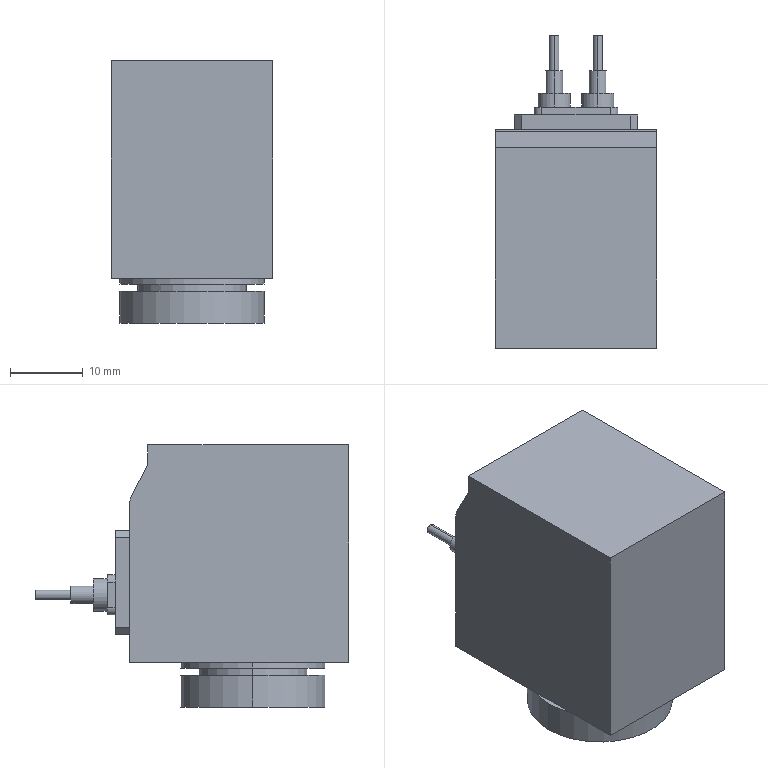Part | SolidWorks | features BaseBody 1 | 1 solid | 54 faces | box 22.3 x 43.2 x 36.2 mm | volume 22382 mm3 | plane 31 | cylinder 23 | commonest cylinder face diameters 1.3 x4 2 x4 2.4 x4 4.5 x4 20 x4 15 x2
STEP:
#1=CARTESIAN_POINT('',(-10.,0.,-31.8));
#2=VERTEX_POINT('',#1);
#3=CARTESIAN_POINT('',(10.,0.,-31.8));
#4=VERTEX_POINT('',#3);
#5=CARTESIAN_POINT('',(0.,0.,-31.8));
#6=DIRECTION('',(0.,0.,-1.));
#7=DIRECTION('',(-1.,0.,0.));
#8=AXIS2_PLACEMENT_3D('',#5,#6,#7);
#9=CIRCLE('',#8,10.);
#10=EDGE_CURVE('',#2,#4,#9,.T.);
#11=ORIENTED_EDGE('',*,*,#10,.T.);
#12=CARTESIAN_POINT('',(10.,0.,-36.2));
#13=VERTEX_POINT('',#12);
#14=CARTESIAN_POINT('',(10.,0.,-36.2));
#15=DIRECTION('',(0.,0.,-1.));
#16=VECTOR('',#15,1000.);
#17=LINE('',#14,#16);
#18=EDGE_CURVE('',#4,#13,#17,.T.);
#19=ORIENTED_EDGE('',*,*,#18,.T.);
#20=CARTESIAN_POINT('',(-10.,0.,-36.2));
#21=VERTEX_POINT('',#20);
#22=CARTESIAN_POINT('',(0.,0.,-36.2));
#23=DIRECTION('',(0.,0.,-1.));
#24=DIRECTION('',(-1.,0.,0.));
#25=AXIS2_PLACEMENT_3D('',#22,#23,#24);
#26=CIRCLE('',#25,10.);
#27=EDGE_CURVE('',#21,#13,#26,.T.);
#28=ORIENTED_EDGE('',*,*,#27,.F.);
#29=CARTESIAN_POINT('',(-10.,0.,-36.2));
#30=DIRECTION('',(0.,0.,-1.));
#31=VECTOR('',#30,1000.);
#32=LINE('',#29,#31);
#33=EDGE_CURVE('',#2,#21,#32,.T.);
#34=ORIENTED_EDGE('',*,*,#33,.F.);
#35=EDGE_LOOP('',(#11,#19,#28,#34));
#36=FACE_OUTER_BOUND('',#35,.T.);
#37=CARTESIAN_POINT('',(0.,0.,-36.2));
#38=DIRECTION('',(0.,0.,-1.));
#39=DIRECTION('',(-1.,0.,0.));
#40=AXIS2_PLACEMENT_3D('',#37,#38,#39);
#41=CYLINDRICAL_SURFACE('',#40,10.);
#42=ADVANCED_FACE('',(#36),#41,.T.);
#43=CARTESIAN_POINT('',(-3.,30.,-20.05));
#44=VERTEX_POINT('',#43);
#45=CARTESIAN_POINT('',(-3.,30.,-21.35));
#46=VERTEX_POINT('',#45);
#47=CARTESIAN_POINT('',(-3.,30.,-20.7));
#48=DIRECTION('',(0.,1.,0.));
#49=DIRECTION('',(1.,0.,0.));
#50=AXIS2_PLACEMENT_3D('',#47,#48,#49);
#51=CIRCLE('',#50,0.65);
#52=EDGE_CURVE('',#44,#46,#51,.T.);
#53=ORIENTED_EDGE('',*,*,#52,.F.);
#54=CARTESIAN_POINT('',(-3.,25.1,-20.05));
#55=VERTEX_POINT('',#54);
#56=CARTESIAN_POINT('',(-3.,30.,-20.05));
#57=DIRECTION('',(0.,-1.,0.));
#58=VECTOR('',#57,1000.);
#59=LINE('',#56,#58);
#60=EDGE_CURVE('',#44,#55,#59,.T.);
#61=ORIENTED_EDGE('',*,*,#60,.T.);
#62=CARTESIAN_POINT('',(-3.,25.1,-21.35));
#63=VERTEX_POINT('',#62);
#64=CARTESIAN_POINT('',(-3.,25.1,-20.7));
#65=DIRECTION('',(0.,1.,0.));
#66=DIRECTION('',(1.,0.,0.));
#67=AXIS2_PLACEMENT_3D('',#64,#65,#66);
#68=CIRCLE('',#67,0.65);
#69=EDGE_CURVE('',#55,#63,#68,.T.);
#70=ORIENTED_EDGE('',*,*,#69,.T.);
#71=CARTESIAN_POINT('',(-3.,30.,-21.35));
#72=DIRECTION('',(0.,-1.,0.));
#73=VECTOR('',#72,1000.);
#74=LINE('',#71,#73);
#75=EDGE_CURVE('',#46,#63,#74,.T.);
#76=ORIENTED_EDGE('',*,*,#75,.F.);
#77=EDGE_LOOP('',(#53,#61,#70,#76));
#78=FACE_OUTER_BOUND('',#77,.T.);
#79=CARTESIAN_POINT('',(-3.,30.,-20.7));
#80=DIRECTION('',(0.,-1.,0.));
#81=DIRECTION('',(0.,0.,-1.));
#82=AXIS2_PLACEMENT_3D('',#79,#80,#81);
#83=CYLINDRICAL_SURFACE('',#82,0.65);
#84=ADVANCED_FACE('',(#78),#83,.T.);
#85=CARTESIAN_POINT('',(3.,30.,-20.05));
#86=VERTEX_POINT('',#85);
#87=CARTESIAN_POINT('',(3.,30.,-21.35));
#88=VERTEX_POINT('',#87);
#89=CARTESIAN_POINT('',(3.,30.,-20.7));
#90=DIRECTION('',(0.,1.,0.));
#91=DIRECTION('',(1.,0.,0.));
#92=AXIS2_PLACEMENT_3D('',#89,#90,#91);
#93=CIRCLE('',#92,0.65);
#94=EDGE_CURVE('',#86,#88,#93,.T.);
#95=ORIENTED_EDGE('',*,*,#94,.F.);
#96=CARTESIAN_POINT('',(3.,25.1,-20.05));
#97=VERTEX_POINT('',#96);
#98=CARTESIAN_POINT('',(3.,30.,-20.05));
#99=DIRECTION('',(0.,-1.,0.));
#100=VECTOR('',#99,1000.);
#101=LINE('',#98,#100);
#102=EDGE_CURVE('',#86,#97,#101,.T.);
#103=ORIENTED_EDGE('',*,*,#102,.T.);
#104=CARTESIAN_POINT('',(3.,25.1,-21.35));
#105=VERTEX_POINT('',#104);
#106=CARTESIAN_POINT('',(3.,25.1,-20.7));
#107=DIRECTION('',(0.,1.,0.));
#108=DIRECTION('',(1.,0.,0.));
#109=AXIS2_PLACEMENT_3D('',#106,#107,#108);
#110=CIRCLE('',#109,0.65);
#111=EDGE_CURVE('',#97,#105,#110,.T.);
#112=ORIENTED_EDGE('',*,*,#111,.T.);
#113=CARTESIAN_POINT('',(3.,30.,-21.35));
#114=DIRECTION('',(0.,-1.,0.));
#115=VECTOR('',#114,1000.);
#116=LINE('',#113,#115);
#117=EDGE_CURVE('',#88,#105,#116,.T.);
#118=ORIENTED_EDGE('',*,*,#117,.F.);
#119=EDGE_LOOP('',(#95,#103,#112,#118));
#120=FACE_OUTER_BOUND('',#119,.T.);
#121=CARTESIAN_POINT('',(3.,30.,-20.7));
#122=DIRECTION('',(0.,-1.,0.));
#123=DIRECTION('',(0.,0.,-1.));
#124=AXIS2_PLACEMENT_3D('',#121,#122,#123);
#125=CYLINDRICAL_SURFACE('',#124,0.65);
#126=ADVANCED_FACE('',(#120),#125,.T.);
#127=CARTESIAN_POINT('',(-7.5,0.,-30.8));
#128=VERTEX_POINT('',#127);
#129=CARTESIAN_POINT('',(7.5,0.,-30.8));
#130=VERTEX_POINT('',#129);
#131=CARTESIAN_POINT('',(0.,0.,-30.8));
#132=DIRECTION('',(0.,0.,-1.));
#133=DIRECTION('',(-1.,0.,0.));
#134=AXIS2_PLACEMENT_3D('',#131,#132,#133);
#135=CIRCLE('',#134,7.5);
#136=EDGE_CURVE('',#128,#130,#135,.T.);
#137=ORIENTED_EDGE('',*,*,#136,.T.);
#138=CARTESIAN_POINT('',(7.5,0.,-31.8));
#139=VERTEX_POINT('',#138);
#140=CARTESIAN_POINT('',(7.5,0.,-36.2));
#141=DIRECTION('',(0.,0.,-1.));
#142=VECTOR('',#141,1000.);
#143=LINE('',#140,#142);
#144=EDGE_CURVE('',#130,#139,#143,.T.);
#145=ORIENTED_EDGE('',*,*,#144,.T.);
#146=CARTESIAN_POINT('',(-7.5,0.,-31.8));
#147=VERTEX_POINT('',#146);
#148=CARTESIAN_POINT('',(0.,0.,-31.8));
#149=DIRECTION('',(0.,0.,-1.));
#150=DIRECTION('',(-1.,0.,0.));
#151=AXIS2_PLACEMENT_3D('',#148,#149,#150);
#152=CIRCLE('',#151,7.5);
#153=EDGE_CURVE('',#147,#139,#152,.T.);
#154=ORIENTED_EDGE('',*,*,#153,.F.);
#155=CARTESIAN_POINT('',(-7.5,0.,-36.2));
#156=DIRECTION('',(0.,0.,-1.));
#157=VECTOR('',#156,1000.);
#158=LINE('',#155,#157);
#159=EDGE_CURVE('',#128,#147,#158,.T.);
#160=ORIENTED_EDGE('',*,*,#159,.F.);
#161=EDGE_LOOP('',(#137,#145,#154,#160));
#162=FACE_OUTER_BOUND('',#161,.T.);
#163=CARTESIAN_POINT('',(0.,0.,-36.2));
#164=DIRECTION('',(0.,0.,-1.));
#165=DIRECTION('',(-1.,0.,0.));
#166=AXIS2_PLACEMENT_3D('',#163,#164,#165);
#167=CYLINDRICAL_SURFACE('',#166,7.5);
#168=ADVANCED_FACE('',(#162),#167,.T.);
#169=CARTESIAN_POINT('',(-3.,25.1,-19.5));
#170=VERTEX_POINT('',#169);
#171=CARTESIAN_POINT('',(-3.,25.1,-21.9));
#172=VERTEX_POINT('',#171);
#173=CARTESIAN_POINT('',(-3.,25.1,-20.7));
#174=DIRECTION('',(0.,1.,0.));
#175=DIRECTION('',(1.,0.,0.));
#176=AXIS2_PLACEMENT_3D('',#173,#174,#175);
#177=CIRCLE('',#176,1.2);
#178=EDGE_CURVE('',#170,#172,#177,.T.);
#179=ORIENTED_EDGE('',*,*,#178,.F.);
#180=CARTESIAN_POINT('',(-3.,22.,-19.5));
#181=VERTEX_POINT('',#180);
#182=CARTESIAN_POINT('',(-3.,25.1,-19.5));
#183=DIRECTION('',(0.,-1.,0.));
#184=VECTOR('',#183,1000.);
#185=LINE('',#182,#184);
#186=EDGE_CURVE('',#170,#181,#185,.T.);
#187=ORIENTED_EDGE('',*,*,#186,.T.);
#188=CARTESIAN_POINT('',(-3.,22.,-21.9));
#189=VERTEX_POINT('',#188);
#190=CARTESIAN_POINT('',(-3.,22.,-20.7));
#191=DIRECTION('',(0.,-1.,0.));
#192=DIRECTION('',(0.,0.,1.));
#193=AXIS2_PLACEMENT_3D('',#190,#191,#192);
#194=CIRCLE('',#193,1.2);
#195=EDGE_CURVE('',#189,#181,#194,.T.);
#196=ORIENTED_EDGE('',*,*,#195,.F.);
#197=CARTESIAN_POINT('',(-3.,25.1,-21.9));
#198=DIRECTION('',(0.,-1.,0.));
#199=VECTOR('',#198,1000.);
#200=LINE('',#197,#199);
#201=EDGE_CURVE('',#172,#189,#200,.T.);
#202=ORIENTED_EDGE('',*,*,#201,.F.);
#203=EDGE_LOOP('',(#179,#187,#196,#202));
#204=FACE_OUTER_BOUND('',#203,.T.);
#205=CARTESIAN_POINT('',(-3.,25.1,-20.7));
#206=DIRECTION('',(0.,-1.,0.));
#207=DIRECTION('',(0.,0.,-1.));
#208=AXIS2_PLACEMENT_3D('',#205,#206,#207);
#209=CYLINDRICAL_SURFACE('',#208,1.2);
#210=ADVANCED_FACE('',(#204),#209,.T.);
#211=CARTESIAN_POINT('',(3.,25.1,-19.5));
#212=VERTEX_POINT('',#211);
#213=CARTESIAN_POINT('',(3.,25.1,-21.9));
#214=VERTEX_POINT('',#213);
#215=CARTESIAN_POINT('',(3.,25.1,-20.7));
#216=DIRECTION('',(0.,1.,0.));
#217=DIRECTION('',(1.,0.,0.));
#218=AXIS2_PLACEMENT_3D('',#215,#216,#217);
#219=CIRCLE('',#218,1.2);
#220=EDGE_CURVE('',#212,#214,#219,.T.);
#221=ORIENTED_EDGE('',*,*,#220,.F.);
#222=CARTESIAN_POINT('',(3.,22.,-19.5));
#223=VERTEX_POINT('',#222);
#224=CARTESIAN_POINT('',(3.,25.1,-19.5));
#225=DIRECTION('',(0.,-1.,0.));
#226=VECTOR('',#225,1000.);
#227=LINE('',#224,#226);
#228=EDGE_CURVE('',#212,#223,#227,.T.);
#229=ORIENTED_EDGE('',*,*,#228,.T.);
#230=CARTESIAN_POINT('',(3.,22.,-21.9));
#231=VERTEX_POINT('',#230);
#232=CARTESIAN_POINT('',(3.,22.,-20.7));
#233=DIRECTION('',(0.,-1.,0.));
#234=DIRECTION('',(0.,0.,1.));
#235=AXIS2_PLACEMENT_3D('',#232,#233,#234);
#236=CIRCLE('',#235,1.2);
#237=EDGE_CURVE('',#231,#223,#236,.T.);
#238=ORIENTED_EDGE('',*,*,#237,.F.);
#239=CARTESIAN_POINT('',(3.,25.1,-21.9));
#240=DIRECTION('',(0.,-1.,0.));
#241=VECTOR('',#240,1000.);
#242=LINE('',#239,#241);
#243=EDGE_CURVE('',#214,#231,#242,.T.);
#244=ORIENTED_EDGE('',*,*,#243,.F.);
#245=EDGE_LOOP('',(#221,#229,#238,#244));
#246=FACE_OUTER_BOUND('',#245,.T.);
#247=CARTESIAN_POINT('',(3.,25.1,-20.7));
#248=DIRECTION('',(0.,-1.,0.));
#249=DIRECTION('',(0.,0.,-1.));
#250=AXIS2_PLACEMENT_3D('',#247,#248,#249);
#251=CYLINDRICAL_SURFACE('',#250,1.2);
#252=ADVANCED_FACE('',(#246),#251,.T.);
#253=CARTESIAN_POINT('',(-10.,0.,-30.));
#254=VERTEX_POINT('',#253);
#255=CARTESIAN_POINT('',(10.,0.,-30.));
#256=VERTEX_POINT('',#255);
#257=CARTESIAN_POINT('',(0.,0.,-30.));
#258=DIRECTION('',(0.,0.,-1.));
#259=DIRECTION('',(1.,0.,0.));
#260=AXIS2_PLACEMENT_3D('',#257,#258,#259);
#261=CIRCLE('',#260,10.);
#262=EDGE_CURVE('',#254,#256,#261,.T.);
#263=ORIENTED_EDGE('',*,*,#262,.T.);
#264=CARTESIAN_POINT('',(10.,0.,-30.8));
#265=VERTEX_POINT('',#264);
#266=CARTESIAN_POINT('',(10.,0.,-36.2));
#267=DIRECTION('',(0.,0.,-1.));
#268=VECTOR('',#267,1000.);
#269=LINE('',#266,#268);
#270=EDGE_CURVE('',#256,#265,#269,.T.);
#271=ORIENTED_EDGE('',*,*,#270,.T.);
#272=CARTESIAN_POINT('',(-10.,0.,-30.8));
#273=VERTEX_POINT('',#272);
#274=CARTESIAN_POINT('',(0.,0.,-30.8));
#275=DIRECTION('',(0.,0.,-1.));
#276=DIRECTION('',(-1.,0.,0.));
#277=AXIS2_PLACEMENT_3D('',#274,#275,#276);
#278=CIRCLE('',#277,10.);
#279=EDGE_CURVE('',#273,#265,#278,.T.);
#280=ORIENTED_EDGE('',*,*,#279,.F.);
#281=CARTESIAN_POINT('',(-10.,0.,-36.2));
#282=DIRECTION('',(0.,0.,-1.));
#283=VECTOR('',#282,1000.);
#284=LINE('',#281,#283);
#285=EDGE_CURVE('',#254,#273,#284,.T.);
#286=ORIENTED_EDGE('',*,*,#285,.F.);
#287=EDGE_LOOP('',(#263,#271,#280,#286));
#288=FACE_OUTER_BOUND('',#287,.T.);
#289=CARTESIAN_POINT('',(0.,0.,-36.2));
#290=DIRECTION('',(0.,0.,-1.));
#291=DIRECTION('',(-1.,0.,0.));
#292=AXIS2_PLACEMENT_3D('',#289,#290,#291);
#293=CYLINDRICAL_SURFACE('',#292,10.);
#294=ADVANCED_FACE('',(#288),#293,.T.);
#295=CARTESIAN_POINT('',(-3.,22.,-18.45));
#296=VERTEX_POINT('',#295);
#297=CARTESIAN_POINT('',(-3.,22.,-22.95));
#298=VERTEX_POINT('',#297);
#299=CARTESIAN_POINT('',(-3.,22.,-20.7));
#300=DIRECTION('',(0.,1.,0.));
#301=DIRECTION('',(1.,0.,0.));
#302=AXIS2_PLACEMENT_3D('',#299,#300,#301);
#303=CIRCLE('',#302,2.25);
#304=EDGE_CURVE('',#296,#298,#303,.T.);
#305=ORIENTED_EDGE('',*,*,#304,.F.);
#306=CARTESIAN_POINT('',(-3.,20.1,-18.45));
#307=VERTEX_POINT('',#306);
#308=CARTESIAN_POINT('',(-3.,22.,-18.45));
#309=DIRECTION('',(0.,-1.,0.));
#310=VECTOR('',#309,1000.);
#311=LINE('',#308,#310);
#312=EDGE_CURVE('',#296,#307,#311,.T.);
#313=ORIENTED_EDGE('',*,*,#312,.T.);
#314=CARTESIAN_POINT('',(-3.,20.1,-22.95));
#315=VERTEX_POINT('',#314);
#316=CARTESIAN_POINT('',(-3.,20.1,-20.7));
#317=DIRECTION('',(0.,1.,0.));
#318=DIRECTION('',(1.,0.,0.));
#319=AXIS2_PLACEMENT_3D('',#316,#317,#318);
#320=CIRCLE('',#319,2.25);
#321=EDGE_CURVE('',#307,#315,#320,.T.);
#322=ORIENTED_EDGE('',*,*,#321,.T.);
#323=CARTESIAN_POINT('',(-3.,22.,-22.95));
#324=DIRECTION('',(0.,-1.,0.));
#325=VECTOR('',#324,1000.);
#326=LINE('',#323,#325);
#327=EDGE_CURVE('',#298,#315,#326,.T.);
#328=ORIENTED_EDGE('',*,*,#327,.F.);
#329=EDGE_LOOP('',(#305,#313,#322,#328));
#330=FACE_OUTER_BOUND('',#329,.T.);
#331=CARTESIAN_POINT('',(-3.,22.,-20.7));
#332=DIRECTION('',(0.,-1.,0.));
#333=DIRECTION('',(0.,0.,-1.));
#334=AXIS2_PLACEMENT_3D('',#331,#332,#333);
#335=CYLINDRICAL_SURFACE('',#334,2.25);
#336=ADVANCED_FACE('',(#330),#335,.T.);
#337=CARTESIAN_POINT('',(3.,22.,-18.45));
#338=VERTEX_POINT('',#337);
#339=CARTESIAN_POINT('',(3.,22.,-22.95));
#340=VERTEX_POINT('',#339);
#341=CARTESIAN_POINT('',(3.,22.,-20.7));
#342=DIRECTION('',(0.,1.,0.));
#343=DIRECTION('',(1.,0.,0.));
#344=AXIS2_PLACEMENT_3D('',#341,#342,#343);
#345=CIRCLE('',#344,2.25);
#346=EDGE_CURVE('',#338,#340,#345,.T.);
#347=ORIENTED_EDGE('',*,*,#346,.F.);
#348=CARTESIAN_POINT('',(3.,20.1,-18.45));
#349=VERTEX_POINT('',#348);
#350=CARTESIAN_POINT('',(3.,22.,-18.45));
#351=DIRECTION('',(0.,-1.,0.));
#352=VECTOR('',#351,1000.);
#353=LINE('',#350,#352);
#354=EDGE_CURVE('',#338,#349,#353,.T.);
#355=ORIENTED_EDGE('',*,*,#354,.T.);
#356=CARTESIAN_POINT('',(3.,20.1,-22.95));
#357=VERTEX_POINT('',#356);
#358=CARTESIAN_POINT('',(3.,20.1,-20.7));
#359=DIRECTION('',(0.,1.,0.));
#360=DIRECTION('',(1.,0.,0.));
#361=AXIS2_PLACEMENT_3D('',#358,#359,#360);
#362=CIRCLE('',#361,2.25);
#363=EDGE_CURVE('',#349,#357,#362,.T.);
#364=ORIENTED_EDGE('',*,*,#363,.T.);
#365=CARTESIAN_POINT('',(3.,22.,-22.95));
#366=DIRECTION('',(0.,-1.,0.));
#367=VECTOR('',#366,1000.);
#368=LINE('',#365,#367);
#369=EDGE_CURVE('',#340,#357,#368,.T.);
#370=ORIENTED_EDGE('',*,*,#369,.F.);
#371=EDGE_LOOP('',(#347,#355,#364,#370));
#372=FACE_OUTER_BOUND('',#371,.T.);
#373=CARTESIAN_POINT('',(3.,22.,-20.7));
#374=DIRECTION('',(0.,-1.,0.));
#375=DIRECTION('',(0.,0.,-1.));
#376=AXIS2_PLACEMENT_3D('',#373,#374,#375);
#377=CYLINDRICAL_SURFACE('',#376,2.25);
#378=ADVANCED_FACE('',(#372),#377,.T.);
#379=CARTESIAN_POINT('',(-7.5,19.,-26.2));
#380=VERTEX_POINT('',#379);
#381=CARTESIAN_POINT('',(-8.5,19.,-25.2));
#382=VERTEX_POINT('',#381);
#383=CARTESIAN_POINT('',(-7.5,19.,-26.2));
#384=DIRECTION('',(-0.7071,0.,0.7071));
#385=VECTOR('',#384,1000.);
#386=LINE('',#383,#385);
#387=EDGE_CURVE('',#380,#382,#386,.T.);
#388=ORIENTED_EDGE('',*,*,#387,.T.);
#389=CARTESIAN_POINT('',(-8.5,19.,-12.8));
#390=VERTEX_POINT('',#389);
#391=CARTESIAN_POINT('',(-8.5,19.,-25.2));
#392=DIRECTION('',(0.,0.,1.));
#393=VECTOR('',#392,1000.);
#394=LINE('',#391,#393);
#395=EDGE_CURVE('',#382,#390,#394,.T.);
#396=ORIENTED_EDGE('',*,*,#395,.T.);
#397=CARTESIAN_POINT('',(-7.5,19.,-11.8));
#398=VERTEX_POINT('',#397);
#399=CARTESIAN_POINT('',(-8.5,19.,-12.8));
#400=DIRECTION('',(0.7071,0.,0.7071));
#401=VECTOR('',#400,1000.);
#402=LINE('',#399,#401);
#403=EDGE_CURVE('',#390,#398,#402,.T.);
#404=ORIENTED_EDGE('',*,*,#403,.T.);
#405=CARTESIAN_POINT('',(7.5,19.,-11.8));
#406=VERTEX_POINT('',#405);
#407=CARTESIAN_POINT('',(-7.5,19.,-11.8));
#408=DIRECTION('',(1.,0.,0.));
#409=VECTOR('',#408,1000.);
#410=LINE('',#407,#409);
#411=EDGE_CURVE('',#398,#406,#410,.T.);
#412=ORIENTED_EDGE('',*,*,#411,.T.);
#413=CARTESIAN_POINT('',(8.5,19.,-12.8));
#414=VERTEX_POINT('',#413);
#415=CARTESIAN_POINT('',(7.5,19.,-11.8));
#416=DIRECTION('',(0.7071,0.,-0.7071));
#417=VECTOR('',#416,1000.);
#418=LINE('',#415,#417);
#419=EDGE_CURVE('',#406,#414,#418,.T.);
#420=ORIENTED_EDGE('',*,*,#419,.T.);
#421=CARTESIAN_POINT('',(8.5,19.,-25.2));
#422=VERTEX_POINT('',#421);
#423=CARTESIAN_POINT('',(8.5,19.,-12.8));
#424=DIRECTION('',(0.,0.,-1.));
#425=VECTOR('',#424,1000.);
#426=LINE('',#423,#425);
#427=EDGE_CURVE('',#414,#422,#426,.T.);
#428=ORIENTED_EDGE('',*,*,#427,.T.);
#429=CARTESIAN_POINT('',(7.5,19.,-26.2));
#430=VERTEX_POINT('',#429);
#431=CARTESIAN_POINT('',(8.5,19.,-25.2));
#432=DIRECTION('',(-0.7071,0.,-0.7071));
#433=VECTOR('',#432,1000.);
#434=LINE('',#431,#433);
#435=EDGE_CURVE('',#422,#430,#434,.T.);
#436=ORIENTED_EDGE('',*,*,#435,.T.);
#437=CARTESIAN_POINT('',(7.5,19.,-26.2));
#438=DIRECTION('',(-1.,0.,0.));
#439=VECTOR('',#438,1000.);
#440=LINE('',#437,#439);
#441=EDGE_CURVE('',#430,#380,#440,.T.);
#442=ORIENTED_EDGE('',*,*,#441,.T.);
#443=EDGE_LOOP('',(#388,#396,#404,#412,#420,#428,#436,#442));
#444=FACE_OUTER_BOUND('',#443,.T.);
#445=CARTESIAN_POINT('',(-5.75,19.,-18.95));
#446=VERTEX_POINT('',#445);
#447=CARTESIAN_POINT('',(-5.75,19.,-22.45));
#448=VERTEX_POINT('',#447);
#449=CARTESIAN_POINT('',(-5.75,19.,-18.95));
#450=DIRECTION('',(0.,0.,-1.));
#451=VECTOR('',#450,1000.);
#452=LINE('',#449,#451);
#453=EDGE_CURVE('',#446,#448,#452,.T.);
#454=ORIENTED_EDGE('',*,*,#453,.T.);
#455=CARTESIAN_POINT('',(-4.75,19.,-23.45));
#456=VERTEX_POINT('',#455);
#457=CARTESIAN_POINT('',(-4.75,19.,-22.45));
#458=DIRECTION('',(0.,-1.,0.));
#459=DIRECTION('',(-1.,0.,0.));
#460=AXIS2_PLACEMENT_3D('',#457,#458,#459);
#461=CIRCLE('',#460,1.);
#462=EDGE_CURVE('',#448,#456,#461,.T.);
#463=ORIENTED_EDGE('',*,*,#462,.T.);
#464=CARTESIAN_POINT('',(4.75,19.,-23.45));
#465=VERTEX_POINT('',#464);
#466=CARTESIAN_POINT('',(-4.75,19.,-23.45));
#467=DIRECTION('',(1.,0.,0.));
#468=VECTOR('',#467,1000.);
#469=LINE('',#466,#468);
#470=EDGE_CURVE('',#456,#465,#469,.T.);
#471=ORIENTED_EDGE('',*,*,#470,.T.);
#472=CARTESIAN_POINT('',(5.75,19.,-22.45));
#473=VERTEX_POINT('',#472);
#474=CARTESIAN_POINT('',(4.75,19.,-22.45));
#475=DIRECTION('',(0.,-1.,0.));
#476=DIRECTION('',(0.,0.,-1.));
#477=AXIS2_PLACEMENT_3D('',#474,#475,#476);
#478=CIRCLE('',#477,1.);
#479=EDGE_CURVE('',#465,#473,#478,.T.);
#480=ORIENTED_EDGE('',*,*,#479,.T.);
#481=CARTESIAN_POINT('',(5.75,19.,-18.95));
#482=VERTEX_POINT('',#481);
#483=CARTESIAN_POINT('',(5.75,19.,-22.45));
#484=DIRECTION('',(0.,0.,1.));
#485=VECTOR('',#484,1000.);
#486=LINE('',#483,#485);
#487=EDGE_CURVE('',#473,#482,#486,.T.);
#488=ORIENTED_EDGE('',*,*,#487,.T.);
#489=CARTESIAN_POINT('',(4.75,19.,-17.95));
#490=VERTEX_POINT('',#489);
#491=CARTESIAN_POINT('',(4.75,19.,-18.95));
#492=DIRECTION('',(0.,-1.,0.));
#493=DIRECTION('',(1.,0.,0.));
#494=AXIS2_PLACEMENT_3D('',#491,#492,#493);
#495=CIRCLE('',#494,1.);
#496=EDGE_CURVE('',#482,#490,#495,.T.);
#497=ORIENTED_EDGE('',*,*,#496,.T.);
#498=CARTESIAN_POINT('',(-4.75,19.,-17.95));
#499=VERTEX_POINT('',#498);
#500=CARTESIAN_POINT('',(4.75,19.,-17.95));
#501=DIRECTION('',(-1.,0.,0.));
#502=VECTOR('',#501,1000.);
#503=LINE('',#500,#502);
#504=EDGE_CURVE('',#490,#499,#503,.T.);
#505=ORIENTED_EDGE('',*,*,#504,.T.);
#506=CARTESIAN_POINT('',(-4.75,19.,-18.95));
#507=DIRECTION('',(0.,-1.,0.));
#508=DIRECTION('',(0.,0.,1.));
#509=AXIS2_PLACEMENT_3D('',#506,#507,#508);
#510=CIRCLE('',#509,1.);
#511=EDGE_CURVE('',#499,#446,#510,.T.);
#512=ORIENTED_EDGE('',*,*,#511,.T.);
#513=EDGE_LOOP('',(#454,#463,#471,#480,#488,#497,#505,#512));
#514=FACE_BOUND('',#513,.T.);
#515=CARTESIAN_POINT('',(0.,19.,0.));
#516=DIRECTION('',(0.,1.,0.));
#517=DIRECTION('',(0.,0.,1.));
#518=AXIS2_PLACEMENT_3D('',#515,#516,#517);
#519=PLANE('',#518);
#520=ADVANCED_FACE('',(#444,#514),#519,.T.);
#521=CARTESIAN_POINT('',(-7.5,17.,-26.2));
#522=VERTEX_POINT('',#521);
#523=CARTESIAN_POINT('',(-8.5,17.,-25.2));
#524=VERTEX_POINT('',#523);
#525=CARTESIAN_POINT('',(-7.5,17.,-26.2));
#526=DIRECTION('',(-0.7071,0.,0.7071));
#527=VECTOR('',#526,1000.);
#528=LINE('',#525,#527);
#529=EDGE_CURVE('',#522,#524,#528,.T.);
#530=ORIENTED_EDGE('',*,*,#529,.T.);
#531=CARTESIAN_POINT('',(-8.5,19.,-25.2));
#532=DIRECTION('',(0.,-1.,0.));
#533=VECTOR('',#532,1000.);
#534=LINE('',#531,#533);
#535=EDGE_CURVE('',#382,#524,#534,.T.);
#536=ORIENTED_EDGE('',*,*,#535,.F.);
#537=ORIENTED_EDGE('',*,*,#387,.F.);
#538=CARTESIAN_POINT('',(-7.5,19.,-26.2));
#539=DIRECTION('',(0.,-1.,0.));
#540=VECTOR('',#539,1000.);
#541=LINE('',#538,#540);
#542=EDGE_CURVE('',#380,#522,#541,.T.);
#543=ORIENTED_EDGE('',*,*,#542,.T.);
#544=EDGE_LOOP('',(#530,#536,#537,#543));
#545=FACE_OUTER_BOUND('',#544,.T.);
#546=CARTESIAN_POINT('',(-7.5,19.,-26.2));
#547=DIRECTION('',(0.7071,0.,0.7071));
#548=DIRECTION('',(0.7071,0.,-0.7071));
#549=AXIS2_PLACEMENT_3D('',#546,#547,#548);
#550=PLANE('',#549);
#551=ADVANCED_FACE('',(#545),#550,.F.);
#552=CARTESIAN_POINT('',(-8.5,17.,-12.8));
#553=VERTEX_POINT('',#552);
#554=CARTESIAN_POINT('',(-8.5,17.,-25.2));
#555=DIRECTION('',(0.,0.,1.));
#556=VECTOR('',#555,1000.);
#557=LINE('',#554,#556);
#558=EDGE_CURVE('',#524,#553,#557,.T.);
#559=ORIENTED_EDGE('',*,*,#558,.T.);
#560=CARTESIAN_POINT('',(-8.5,19.,-12.8));
#561=DIRECTION('',(0.,-1.,0.));
#562=VECTOR('',#561,1000.);
#563=LINE('',#560,#562);
#564=EDGE_CURVE('',#390,#553,#563,.T.);
#565=ORIENTED_EDGE('',*,*,#564,.F.);
#566=ORIENTED_EDGE('',*,*,#395,.F.);
#567=ORIENTED_EDGE('',*,*,#535,.T.);
#568=EDGE_LOOP('',(#559,#565,#566,#567));
#569=FACE_OUTER_BOUND('',#568,.T.);
#570=CARTESIAN_POINT('',(-8.5,19.,-25.2));
#571=DIRECTION('',(1.,0.,0.));
#572=DIRECTION('',(0.,0.,-1.));
#573=AXIS2_PLACEMENT_3D('',#570,#571,#572);
#574=PLANE('',#573);
#575=ADVANCED_FACE('',(#569),#574,.F.);
#576=CARTESIAN_POINT('',(-7.5,17.,-11.8));
#577=VERTEX_POINT('',#576);
#578=CARTESIAN_POINT('',(-8.5,17.,-12.8));
#579=DIRECTION('',(0.7071,0.,0.7071));
#580=VECTOR('',#579,1000.);
#581=LINE('',#578,#580);
#582=EDGE_CURVE('',#553,#577,#581,.T.);
#583=ORIENTED_EDGE('',*,*,#582,.T.);
#584=CARTESIAN_POINT('',(-7.5,19.,-11.8));
#585=DIRECTION('',(0.,-1.,0.));
#586=VECTOR('',#585,1000.);
#587=LINE('',#584,#586);
#588=EDGE_CURVE('',#398,#577,#587,.T.);
#589=ORIENTED_EDGE('',*,*,#588,.F.);
#590=ORIENTED_EDGE('',*,*,#403,.F.);
#591=ORIENTED_EDGE('',*,*,#564,.T.);
#592=EDGE_LOOP('',(#583,#589,#590,#591));
#593=FACE_OUTER_BOUND('',#592,.T.);
#594=CARTESIAN_POINT('',(-8.5,19.,-12.8));
#595=DIRECTION('',(0.7071,0.,-0.7071));
#596=DIRECTION('',(-0.7071,0.,-0.7071));
#597=AXIS2_PLACEMENT_3D('',#594,#595,#596);
#598=PLANE('',#597);
#599=ADVANCED_FACE('',(#593),#598,.F.);
#600=CARTESIAN_POINT('',(7.5,17.,-11.8));
#601=VERTEX_POINT('',#600);
#602=CARTESIAN_POINT('',(-7.5,17.,-11.8));
#603=DIRECTION('',(1.,0.,0.));
#604=VECTOR('',#603,1000.);
#605=LINE('',#602,#604);
#606=EDGE_CURVE('',#577,#601,#605,.T.);
#607=ORIENTED_EDGE('',*,*,#606,.T.);
#608=CARTESIAN_POINT('',(7.5,19.,-11.8));
#609=DIRECTION('',(0.,-1.,0.));
#610=VECTOR('',#609,1000.);
#611=LINE('',#608,#610);
#612=EDGE_CURVE('',#406,#601,#611,.T.);
#613=ORIENTED_EDGE('',*,*,#612,.F.);
#614=ORIENTED_EDGE('',*,*,#411,.F.);
#615=ORIENTED_EDGE('',*,*,#588,.T.);
#616=EDGE_LOOP('',(#607,#613,#614,#615));
#617=FACE_OUTER_BOUND('',#616,.T.);
#618=CARTESIAN_POINT('',(-7.5,19.,-11.8));
#619=DIRECTION('',(0.,0.,-1.));
#620=DIRECTION('',(-1.,0.,0.));
#621=AXIS2_PLACEMENT_3D('',#618,#619,#620);
#622=PLANE('',#621);
#623=ADVANCED_FACE('',(#617),#622,.F.);
#624=CARTESIAN_POINT('',(8.5,17.,-12.8));
#625=VERTEX_POINT('',#624);
#626=CARTESIAN_POINT('',(7.5,17.,-11.8));
#627=DIRECTION('',(0.7071,0.,-0.7071));
#628=VECTOR('',#627,1000.);
#629=LINE('',#626,#628);
#630=EDGE_CURVE('',#601,#625,#629,.T.);
#631=ORIENTED_EDGE('',*,*,#630,.T.);
#632=CARTESIAN_POINT('',(8.5,19.,-12.8));
#633=DIRECTION('',(0.,-1.,0.));
#634=VECTOR('',#633,1000.);
#635=LINE('',#632,#634);
#636=EDGE_CURVE('',#414,#625,#635,.T.);
#637=ORIENTED_EDGE('',*,*,#636,.F.);
#638=ORIENTED_EDGE('',*,*,#419,.F.);
#639=ORIENTED_EDGE('',*,*,#612,.T.);
#640=EDGE_LOOP('',(#631,#637,#638,#639));
#641=FACE_OUTER_BOUND('',#640,.T.);
#642=CARTESIAN_POINT('',(7.5,19.,-11.8));
#643=DIRECTION('',(-0.7071,0.,-0.7071));
#644=DIRECTION('',(-0.7071,0.,0.7071));
#645=AXIS2_PLACEMENT_3D('',#642,#643,#644);
#646=PLANE('',#645);
#647=ADVANCED_FACE('',(#641),#646,.F.);
#648=CARTESIAN_POINT('',(8.5,17.,-25.2));
#649=VERTEX_POINT('',#648);
#650=CARTESIAN_POINT('',(8.5,17.,-12.8));
#651=DIRECTION('',(0.,0.,-1.));
#652=VECTOR('',#651,1000.);
#653=LINE('',#650,#652);
#654=EDGE_CURVE('',#625,#649,#653,.T.);
#655=ORIENTED_EDGE('',*,*,#654,.T.);
#656=CARTESIAN_POINT('',(8.5,19.,-25.2));
#657=DIRECTION('',(0.,-1.,0.));
#658=VECTOR('',#657,1000.);
#659=LINE('',#656,#658);
#660=EDGE_CURVE('',#422,#649,#659,.T.);
#661=ORIENTED_EDGE('',*,*,#660,.F.);
#662=ORIENTED_EDGE('',*,*,#427,.F.);
#663=ORIENTED_EDGE('',*,*,#636,.T.);
#664=EDGE_LOOP('',(#655,#661,#662,#663));
#665=FACE_OUTER_BOUND('',#664,.T.);
#666=CARTESIAN_POINT('',(8.5,19.,-12.8));
#667=DIRECTION('',(-1.,0.,0.));
#668=DIRECTION('',(0.,0.,1.));
#669=AXIS2_PLACEMENT_3D('',#666,#667,#668);
#670=PLANE('',#669);
#671=ADVANCED_FACE('',(#665),#670,.F.);
#672=CARTESIAN_POINT('',(7.5,17.,-26.2));
#673=VERTEX_POINT('',#672);
#674=CARTESIAN_POINT('',(8.5,17.,-25.2));
#675=DIRECTION('',(-0.7071,0.,-0.7071));
#676=VECTOR('',#675,1000.);
#677=LINE('',#674,#676);
#678=EDGE_CURVE('',#649,#673,#677,.T.);
#679=ORIENTED_EDGE('',*,*,#678,.T.);
#680=CARTESIAN_POINT('',(7.5,19.,-26.2));
#681=DIRECTION('',(0.,-1.,0.));
#682=VECTOR('',#681,1000.);
#683=LINE('',#680,#682);
#684=EDGE_CURVE('',#430,#673,#683,.T.);
#685=ORIENTED_EDGE('',*,*,#684,.F.);
#686=ORIENTED_EDGE('',*,*,#435,.F.);
#687=ORIENTED_EDGE('',*,*,#660,.T.);
#688=EDGE_LOOP('',(#679,#685,#686,#687));
#689=FACE_OUTER_BOUND('',#688,.T.);
#690=CARTESIAN_POINT('',(8.5,19.,-25.2));
#691=DIRECTION('',(-0.7071,0.,0.7071));
#692=DIRECTION('',(0.7071,0.,0.7071));
#693=AXIS2_PLACEMENT_3D('',#690,#691,#692);
#694=PLANE('',#693);
#695=ADVANCED_FACE('',(#689),#694,.F.);
#696=CARTESIAN_POINT('',(7.5,17.,-26.2));
#697=DIRECTION('',(-1.,0.,0.));
#698=VECTOR('',#697,1000.);
#699=LINE('',#696,#698);
#700=EDGE_CURVE('',#673,#522,#699,.T.);
#701=ORIENTED_EDGE('',*,*,#700,.T.);
#702=ORIENTED_EDGE('',*,*,#542,.F.);
#703=ORIENTED_EDGE('',*,*,#441,.F.);
#704=ORIENTED_EDGE('',*,*,#684,.T.);
#705=EDGE_LOOP('',(#701,#702,#703,#704));
#706=FACE_OUTER_BOUND('',#705,.T.);
#707=CARTESIAN_POINT('',(7.5,19.,-26.2));
#708=DIRECTION('',(0.,0.,1.));
#709=DIRECTION('',(1.,0.,0.));
#710=AXIS2_PLACEMENT_3D('',#707,#708,#709);
#711=PLANE('',#710);
#712=ADVANCED_FACE('',(#706),#711,.F.);
#713=ORIENTED_EDGE('',*,*,#453,.F.);
#714=CARTESIAN_POINT('',(-5.75,20.1,-18.95));
#715=VERTEX_POINT('',#714);
#716=CARTESIAN_POINT('',(-5.75,20.1,-18.95));
#717=DIRECTION('',(0.,-1.,0.));
#718=VECTOR('',#717,1000.);
#719=LINE('',#716,#718);
#720=EDGE_CURVE('',#715,#446,#719,.T.);
#721=ORIENTED_EDGE('',*,*,#720,.F.);
#722=CARTESIAN_POINT('',(-5.75,20.1,-22.45));
#723=VERTEX_POINT('',#722);
#724=CARTESIAN_POINT('',(-5.75,20.1,-22.45));
#725=DIRECTION('',(0.,0.,1.));
#726=VECTOR('',#725,1000.);
#727=LINE('',#724,#726);
#728=EDGE_CURVE('',#723,#715,#727,.T.);
#729=ORIENTED_EDGE('',*,*,#728,.F.);
#730=CARTESIAN_POINT('',(-5.75,20.1,-22.45));
#731=DIRECTION('',(0.,-1.,0.));
#732=VECTOR('',#731,1000.);
#733=LINE('',#730,#732);
#734=EDGE_CURVE('',#723,#448,#733,.T.);
#735=ORIENTED_EDGE('',*,*,#734,.T.);
#736=EDGE_LOOP('',(#713,#721,#729,#735));
#737=FACE_OUTER_BOUND('',#736,.T.);
#738=CARTESIAN_POINT('',(-5.75,20.1,-22.45));
#739=DIRECTION('',(1.,0.,0.));
#740=DIRECTION('',(0.,0.,-1.));
#741=AXIS2_PLACEMENT_3D('',#738,#739,#740);
#742=PLANE('',#741);
#743=ADVANCED_FACE('',(#737),#742,.F.);
#744=ORIENTED_EDGE('',*,*,#462,.F.);
#745=ORIENTED_EDGE('',*,*,#734,.F.);
#746=CARTESIAN_POINT('',(-4.75,20.1,-23.45));
#747=VERTEX_POINT('',#746);
#748=CARTESIAN_POINT('',(-4.75,20.1,-22.45));
#749=DIRECTION('',(0.,1.,0.));
#750=DIRECTION('',(0.,0.,-1.));
#751=AXIS2_PLACEMENT_3D('',#748,#749,#750);
#752=CIRCLE('',#751,1.);
#753=EDGE_CURVE('',#747,#723,#752,.T.);
#754=ORIENTED_EDGE('',*,*,#753,.F.);
#755=CARTESIAN_POINT('',(-4.75,20.1,-23.45));
#756=DIRECTION('',(0.,-1.,0.));
#757=VECTOR('',#756,1000.);
#758=LINE('',#755,#757);
#759=EDGE_CURVE('',#747,#456,#758,.T.);
#760=ORIENTED_EDGE('',*,*,#759,.T.);
#761=EDGE_LOOP('',(#744,#745,#754,#760));
#762=FACE_OUTER_BOUND('',#761,.T.);
#763=CARTESIAN_POINT('',(-4.75,20.1,-22.45));
#764=DIRECTION('',(0.,-1.,0.));
#765=DIRECTION('',(0.,0.,-1.));
#766=AXIS2_PLACEMENT_3D('',#763,#764,#765);
#767=CYLINDRICAL_SURFACE('',#766,1.);
#768=ADVANCED_FACE('',(#762),#767,.T.);
#769=ORIENTED_EDGE('',*,*,#470,.F.);
#770=ORIENTED_EDGE('',*,*,#759,.F.);
#771=CARTESIAN_POINT('',(4.75,20.1,-23.45));
#772=VERTEX_POINT('',#771);
#773=CARTESIAN_POINT('',(4.75,20.1,-23.45));
#774=DIRECTION('',(-1.,0.,0.));
#775=VECTOR('',#774,1000.);
#776=LINE('',#773,#775);
#777=EDGE_CURVE('',#772,#747,#776,.T.);
#778=ORIENTED_EDGE('',*,*,#777,.F.);
#779=CARTESIAN_POINT('',(4.75,20.1,-23.45));
#780=DIRECTION('',(0.,-1.,0.));
#781=VECTOR('',#780,1000.);
#782=LINE('',#779,#781);
#783=EDGE_CURVE('',#772,#465,#782,.T.);
#784=ORIENTED_EDGE('',*,*,#783,.T.);
#785=EDGE_LOOP('',(#769,#770,#778,#784));
#786=FACE_OUTER_BOUND('',#785,.T.);
#787=CARTESIAN_POINT('',(4.75,20.1,-23.45));
#788=DIRECTION('',(0.,0.,1.));
#789=DIRECTION('',(1.,0.,0.));
#790=AXIS2_PLACEMENT_3D('',#787,#788,#789);
#791=PLANE('',#790);
#792=ADVANCED_FACE('',(#786),#791,.F.);
#793=ORIENTED_EDGE('',*,*,#479,.F.);
#794=ORIENTED_EDGE('',*,*,#783,.F.);
#795=CARTESIAN_POINT('',(5.75,20.1,-22.45));
#796=VERTEX_POINT('',#795);
#797=CARTESIAN_POINT('',(4.75,20.1,-22.45));
#798=DIRECTION('',(0.,1.,0.));
#799=DIRECTION('',(1.,0.,0.));
#800=AXIS2_PLACEMENT_3D('',#797,#798,#799);
#801=CIRCLE('',#800,1.);
#802=EDGE_CURVE('',#796,#772,#801,.T.);
#803=ORIENTED_EDGE('',*,*,#802,.F.);
#804=CARTESIAN_POINT('',(5.75,20.1,-22.45));
#805=DIRECTION('',(0.,-1.,0.));
#806=VECTOR('',#805,1000.);
#807=LINE('',#804,#806);
#808=EDGE_CURVE('',#796,#473,#807,.T.);
#809=ORIENTED_EDGE('',*,*,#808,.T.);
#810=EDGE_LOOP('',(#793,#794,#803,#809));
#811=FACE_OUTER_BOUND('',#810,.T.);
#812=CARTESIAN_POINT('',(4.75,20.1,-22.45));
#813=DIRECTION('',(0.,-1.,0.));
#814=DIRECTION('',(0.,0.,-1.));
#815=AXIS2_PLACEMENT_3D('',#812,#813,#814);
#816=CYLINDRICAL_SURFACE('',#815,1.);
#817=ADVANCED_FACE('',(#811),#816,.T.);
#818=ORIENTED_EDGE('',*,*,#487,.F.);
#819=ORIENTED_EDGE('',*,*,#808,.F.);
#820=CARTESIAN_POINT('',(5.75,20.1,-18.95));
#821=VERTEX_POINT('',#820);
#822=CARTESIAN_POINT('',(5.75,20.1,-18.95));
#823=DIRECTION('',(0.,0.,-1.));
#824=VECTOR('',#823,1000.);
#825=LINE('',#822,#824);
#826=EDGE_CURVE('',#821,#796,#825,.T.);
#827=ORIENTED_EDGE('',*,*,#826,.F.);
#828=CARTESIAN_POINT('',(5.75,20.1,-18.95));
#829=DIRECTION('',(0.,-1.,0.));
#830=VECTOR('',#829,1000.);
#831=LINE('',#828,#830);
#832=EDGE_CURVE('',#821,#482,#831,.T.);
#833=ORIENTED_EDGE('',*,*,#832,.T.);
#834=EDGE_LOOP('',(#818,#819,#827,#833));
#835=FACE_OUTER_BOUND('',#834,.T.);
#836=CARTESIAN_POINT('',(5.75,20.1,-18.95));
#837=DIRECTION('',(-1.,0.,0.));
#838=DIRECTION('',(0.,0.,1.));
#839=AXIS2_PLACEMENT_3D('',#836,#837,#838);
#840=PLANE('',#839);
#841=ADVANCED_FACE('',(#835),#840,.F.);
#842=ORIENTED_EDGE('',*,*,#496,.F.);
#843=ORIENTED_EDGE('',*,*,#832,.F.);
#844=CARTESIAN_POINT('',(4.75,20.1,-17.95));
#845=VERTEX_POINT('',#844);
#846=CARTESIAN_POINT('',(4.75,20.1,-18.95));
#847=DIRECTION('',(0.,1.,0.));
#848=DIRECTION('',(0.,0.,1.));
#849=AXIS2_PLACEMENT_3D('',#846,#847,#848);
#850=CIRCLE('',#849,1.);
#851=EDGE_CURVE('',#845,#821,#850,.T.);
#852=ORIENTED_EDGE('',*,*,#851,.F.);
#853=CARTESIAN_POINT('',(4.75,20.1,-17.95));
#854=DIRECTION('',(0.,-1.,0.));
#855=VECTOR('',#854,1000.);
#856=LINE('',#853,#855);
#857=EDGE_CURVE('',#845,#490,#856,.T.);
#858=ORIENTED_EDGE('',*,*,#857,.T.);
#859=EDGE_LOOP('',(#842,#843,#852,#858));
#860=FACE_OUTER_BOUND('',#859,.T.);
#861=CARTESIAN_POINT('',(4.75,20.1,-18.95));
#862=DIRECTION('',(0.,-1.,0.));
#863=DIRECTION('',(0.,0.,-1.));
#864=AXIS2_PLACEMENT_3D('',#861,#862,#863);
#865=CYLINDRICAL_SURFACE('',#864,1.);
#866=ADVANCED_FACE('',(#860),#865,.T.);
#867=ORIENTED_EDGE('',*,*,#504,.F.);
#868=ORIENTED_EDGE('',*,*,#857,.F.);
#869=CARTESIAN_POINT('',(-4.75,20.1,-17.95));
#870=VERTEX_POINT('',#869);
#871=CARTESIAN_POINT('',(-4.75,20.1,-17.95));
#872=DIRECTION('',(1.,0.,0.));
#873=VECTOR('',#872,1000.);
#874=LINE('',#871,#873);
#875=EDGE_CURVE('',#870,#845,#874,.T.);
#876=ORIENTED_EDGE('',*,*,#875,.F.);
#877=CARTESIAN_POINT('',(-4.75,20.1,-17.95));
#878=DIRECTION('',(0.,-1.,0.));
#879=VECTOR('',#878,1000.);
#880=LINE('',#877,#879);
#881=EDGE_CURVE('',#870,#499,#880,.T.);
#882=ORIENTED_EDGE('',*,*,#881,.T.);
#883=EDGE_LOOP('',(#867,#868,#876,#882));
#884=FACE_OUTER_BOUND('',#883,.T.);
#885=CARTESIAN_POINT('',(-4.75,20.1,-17.95));
#886=DIRECTION('',(0.,0.,-1.));
#887=DIRECTION('',(-1.,0.,0.));
#888=AXIS2_PLACEMENT_3D('',#885,#886,#887);
#889=PLANE('',#888);
#890=ADVANCED_FACE('',(#884),#889,.F.);
#891=ORIENTED_EDGE('',*,*,#511,.F.);
#892=ORIENTED_EDGE('',*,*,#881,.F.);
#893=CARTESIAN_POINT('',(-4.75,20.1,-18.95));
#894=DIRECTION('',(0.,1.,0.));
#895=DIRECTION('',(-1.,0.,0.));
#896=AXIS2_PLACEMENT_3D('',#893,#894,#895);
#897=CIRCLE('',#896,1.);
#898=EDGE_CURVE('',#715,#870,#897,.T.);
#899=ORIENTED_EDGE('',*,*,#898,.F.);
#900=ORIENTED_EDGE('',*,*,#720,.T.);
#901=EDGE_LOOP('',(#891,#892,#899,#900));
#902=FACE_OUTER_BOUND('',#901,.T.);
#903=CARTESIAN_POINT('',(-4.75,20.1,-18.95));
#904=DIRECTION('',(0.,-1.,0.));
#905=DIRECTION('',(0.,0.,-1.));
#906=AXIS2_PLACEMENT_3D('',#903,#904,#905);
#907=CYLINDRICAL_SURFACE('',#906,1.);
#908=ADVANCED_FACE('',(#902),#907,.T.);
#909=CARTESIAN_POINT('',(-11.15,17.,-30.));
#910=VERTEX_POINT('',#909);
#911=CARTESIAN_POINT('',(-11.15,17.,-8.087));
#912=VERTEX_POINT('',#911);
#913=CARTESIAN_POINT('',(-11.15,17.,-30.));
#914=DIRECTION('',(0.,0.,1.));
#915=VECTOR('',#914,1000.);
#916=LINE('',#913,#915);
#917=EDGE_CURVE('',#910,#912,#916,.T.);
#918=ORIENTED_EDGE('',*,*,#917,.T.);
#919=CARTESIAN_POINT('',(11.15,17.,-8.087));
#920=VERTEX_POINT('',#919);
#921=CARTESIAN_POINT('',(11.15,17.,-8.087));
#922=DIRECTION('',(-1.,0.,0.));
#923=VECTOR('',#922,1000.);
#924=LINE('',#921,#923);
#925=EDGE_CURVE('',#920,#912,#924,.T.);
#926=ORIENTED_EDGE('',*,*,#925,.F.);
#927=CARTESIAN_POINT('',(11.15,17.,-30.));
#928=VERTEX_POINT('',#927);
#929=CARTESIAN_POINT('',(11.15,17.,-30.));
#930=DIRECTION('',(0.,0.,1.));
#931=VECTOR('',#930,1000.);
#932=LINE('',#929,#931);
#933=EDGE_CURVE('',#928,#920,#932,.T.);
#934=ORIENTED_EDGE('',*,*,#933,.F.);
#935=CARTESIAN_POINT('',(11.15,17.,-30.));
#936=DIRECTION('',(-1.,0.,0.));
#937=VECTOR('',#936,1000.);
#938=LINE('',#935,#937);
#939=EDGE_CURVE('',#928,#910,#938,.T.);
#940=ORIENTED_EDGE('',*,*,#939,.T.);
#941=EDGE_LOOP('',(#918,#926,#934,#940));
#942=FACE_OUTER_BOUND('',#941,.T.);
#943=ORIENTED_EDGE('',*,*,#558,.F.);
#944=ORIENTED_EDGE('',*,*,#529,.F.);
#945=ORIENTED_EDGE('',*,*,#700,.F.);
#946=ORIENTED_EDGE('',*,*,#678,.F.);
#947=ORIENTED_EDGE('',*,*,#654,.F.);
#948=ORIENTED_EDGE('',*,*,#630,.F.);
#949=ORIENTED_EDGE('',*,*,#606,.F.);
#950=ORIENTED_EDGE('',*,*,#582,.F.);
#951=EDGE_LOOP('',(#943,#944,#945,#946,#947,#948,#949,#950));
#952=FACE_BOUND('',#951,.T.);
#953=CARTESIAN_POINT('',(11.15,17.,-30.));
#954=DIRECTION('',(0.,1.,0.));
#955=DIRECTION('',(0.,0.,1.));
#956=AXIS2_PLACEMENT_3D('',#953,#954,#955);
#957=PLANE('',#956);
#958=ADVANCED_FACE('',(#942,#952),#957,.T.);
#959=CARTESIAN_POINT('',(3.,20.1,-20.7));
#960=DIRECTION('',(0.,1.,0.));
#961=DIRECTION('',(1.,0.,0.));
#962=AXIS2_PLACEMENT_3D('',#959,#960,#961);
#963=CIRCLE('',#962,2.25);
#964=EDGE_CURVE('',#357,#349,#963,.T.);
#965=ORIENTED_EDGE('',*,*,#964,.F.);
#966=ORIENTED_EDGE('',*,*,#363,.F.);
#967=EDGE_LOOP('',(#965,#966));
#968=FACE_BOUND('',#967,.T.);
#969=CARTESIAN_POINT('',(-3.,20.1,-20.7));
#970=DIRECTION('',(0.,1.,0.));
#971=DIRECTION('',(1.,0.,0.));
#972=AXIS2_PLACEMENT_3D('',#969,#970,#971);
#973=CIRCLE('',#972,2.25);
#974=EDGE_CURVE('',#315,#307,#973,.T.);
#975=ORIENTED_EDGE('',*,*,#974,.F.);
#976=ORIENTED_EDGE('',*,*,#321,.F.);
#977=EDGE_LOOP('',(#975,#976));
#978=FACE_BOUND('',#977,.T.);
#979=ORIENTED_EDGE('',*,*,#753,.T.);
#980=ORIENTED_EDGE('',*,*,#728,.T.);
#981=ORIENTED_EDGE('',*,*,#898,.T.);
#982=ORIENTED_EDGE('',*,*,#875,.T.);
#983=ORIENTED_EDGE('',*,*,#851,.T.);
#984=ORIENTED_EDGE('',*,*,#826,.T.);
#985=ORIENTED_EDGE('',*,*,#802,.T.);
#986=ORIENTED_EDGE('',*,*,#777,.T.);
#987=EDGE_LOOP('',(#979,#980,#981,#982,#983,#984,#985,#986));
#988=FACE_OUTER_BOUND('',#987,.T.);
#989=CARTESIAN_POINT('',(-4.75,20.1,-22.45));
#990=DIRECTION('',(0.,1.,0.));
#991=DIRECTION('',(0.,0.,1.));
#992=AXIS2_PLACEMENT_3D('',#989,#990,#991);
#993=PLANE('',#992);
#994=ADVANCED_FACE('',(#968,#978,#988),#993,.T.);
#995=CARTESIAN_POINT('',(-11.15,14.5,0.));
#996=VERTEX_POINT('',#995);
#997=CARTESIAN_POINT('',(-11.15,-13.2,0.));
#998=VERTEX_POINT('',#997);
#999=CARTESIAN_POINT('',(-11.15,14.5,0.));
#1000=DIRECTION('',(0.,-1.,0.));
#1001=VECTOR('',#1000,1000.);
#1002=LINE('',#999,#1001);
#1003=EDGE_CURVE('',#996,#998,#1002,.T.);
#1004=ORIENTED_EDGE('',*,*,#1003,.F.);
#1005=CARTESIAN_POINT('',(-11.15,14.5,-2.7));
#1006=VERTEX_POINT('',#1005);
#1007=CARTESIAN_POINT('',(-11.15,14.5,0.));
#1008=DIRECTION('',(0.,0.,-1.));
#1009=VECTOR('',#1008,1000.);
#1010=LINE('',#1007,#1009);
#1011=EDGE_CURVE('',#996,#1006,#1010,.T.);
#1012=ORIENTED_EDGE('',*,*,#1011,.T.);
#1013=CARTESIAN_POINT('',(-11.15,16.782,-7.179));
#1014=VERTEX_POINT('',#1013);
#1015=CARTESIAN_POINT('',(-11.15,14.5,-2.7));
#1016=DIRECTION('',(0.,0.454,-0.891));
#1017=VECTOR('',#1016,1000.);
#1018=LINE('',#1015,#1017);
#1019=EDGE_CURVE('',#1006,#1014,#1018,.T.);
#1020=ORIENTED_EDGE('',*,*,#1019,.T.);
#1021=CARTESIAN_POINT('',(-11.15,15.,-8.087));
#1022=DIRECTION('',(1.,0.,0.));
#1023=DIRECTION('',(0.,1.,0.));
#1024=AXIS2_PLACEMENT_3D('',#1021,#1022,#1023);
#1025=CIRCLE('',#1024,2.);
#1026=EDGE_CURVE('',#912,#1014,#1025,.T.);
#1027=ORIENTED_EDGE('',*,*,#1026,.F.);
#1028=ORIENTED_EDGE('',*,*,#917,.F.);
#1029=CARTESIAN_POINT('',(-11.15,-13.2,-30.));
#1030=VERTEX_POINT('',#1029);
#1031=CARTESIAN_POINT('',(-11.15,17.,-30.));
#1032=DIRECTION('',(0.,-1.,0.));
#1033=VECTOR('',#1032,1000.);
#1034=LINE('',#1031,#1033);
#1035=EDGE_CURVE('',#910,#1030,#1034,.T.);
#1036=ORIENTED_EDGE('',*,*,#1035,.T.);
#1037=CARTESIAN_POINT('',(-11.15,-13.2,-30.));
#1038=DIRECTION('',(0.,0.,1.));
#1039=VECTOR('',#1038,1000.);
#1040=LINE('',#1037,#1039);
#1041=EDGE_CURVE('',#1030,#998,#1040,.T.);
#1042=ORIENTED_EDGE('',*,*,#1041,.T.);
#1043=EDGE_LOOP('',(#1004,#1012,#1020,#1027,#1028,#1036,#1042));
#1044=FACE_OUTER_BOUND('',#1043,.T.);
#1045=CARTESIAN_POINT('',(-11.15,17.,-30.));
#1046=DIRECTION('',(-1.,0.,0.));
#1047=DIRECTION('',(0.,0.,1.));
#1048=AXIS2_PLACEMENT_3D('',#1045,#1046,#1047);
#1049=PLANE('',#1048);
#1050=ADVANCED_FACE('',(#1044),#1049,.T.);
#1051=ORIENTED_EDGE('',*,*,#1026,.T.);
#1052=CARTESIAN_POINT('',(11.15,16.782,-7.179));
#1053=VERTEX_POINT('',#1052);
#1054=CARTESIAN_POINT('',(11.15,16.782,-7.179));
#1055=DIRECTION('',(-1.,0.,0.));
#1056=VECTOR('',#1055,1000.);
#1057=LINE('',#1054,#1056);
#1058=EDGE_CURVE('',#1053,#1014,#1057,.T.);
#1059=ORIENTED_EDGE('',*,*,#1058,.F.);
#1060=CARTESIAN_POINT('',(11.15,15.,-8.087));
#1061=DIRECTION('',(-1.,0.,0.));
#1062=DIRECTION('',(0.,0.891,0.454));
#1063=AXIS2_PLACEMENT_3D('',#1060,#1061,#1062);
#1064=CIRCLE('',#1063,2.);
#1065=EDGE_CURVE('',#1053,#920,#1064,.T.);
#1066=ORIENTED_EDGE('',*,*,#1065,.T.);
#1067=ORIENTED_EDGE('',*,*,#925,.T.);
#1068=EDGE_LOOP('',(#1051,#1059,#1066,#1067));
#1069=FACE_OUTER_BOUND('',#1068,.T.);
#1070=CARTESIAN_POINT('',(11.5,15.,-8.087));
#1071=DIRECTION('',(-1.,0.,0.));
#1072=DIRECTION('',(0.,0.,1.));
#1073=AXIS2_PLACEMENT_3D('',#1070,#1071,#1072);
#1074=CYLINDRICAL_SURFACE('',#1073,2.);
#1075=ADVANCED_FACE('',(#1069),#1074,.T.);
#1076=CARTESIAN_POINT('',(11.15,14.5,-2.7));
#1077=VERTEX_POINT('',#1076);
#1078=CARTESIAN_POINT('',(11.15,16.782,-7.179));
#1079=DIRECTION('',(0.,-0.454,0.891));
#1080=VECTOR('',#1079,1000.);
#1081=LINE('',#1078,#1080);
#1082=EDGE_CURVE('',#1053,#1077,#1081,.T.);
#1083=ORIENTED_EDGE('',*,*,#1082,.T.);
#1084=CARTESIAN_POINT('',(11.15,14.5,0.));
#1085=VERTEX_POINT('',#1084);
#1086=CARTESIAN_POINT('',(11.15,14.5,-2.7));
#1087=DIRECTION('',(0.,0.,1.));
#1088=VECTOR('',#1087,1000.);
#1089=LINE('',#1086,#1088);
#1090=EDGE_CURVE('',#1077,#1085,#1089,.T.);
#1091=ORIENTED_EDGE('',*,*,#1090,.T.);
#1092=CARTESIAN_POINT('',(11.15,-13.2,0.));
#1093=VERTEX_POINT('',#1092);
#1094=CARTESIAN_POINT('',(11.15,-13.2,0.));
#1095=DIRECTION('',(0.,1.,0.));
#1096=VECTOR('',#1095,1000.);
#1097=LINE('',#1094,#1096);
#1098=EDGE_CURVE('',#1093,#1085,#1097,.T.);
#1099=ORIENTED_EDGE('',*,*,#1098,.F.);
#1100=CARTESIAN_POINT('',(11.15,-13.2,-30.));
#1101=VERTEX_POINT('',#1100);
#1102=CARTESIAN_POINT('',(11.15,-13.2,-30.));
#1103=DIRECTION('',(0.,0.,1.));
#1104=VECTOR('',#1103,1000.);
#1105=LINE('',#1102,#1104);
#1106=EDGE_CURVE('',#1101,#1093,#1105,.T.);
#1107=ORIENTED_EDGE('',*,*,#1106,.F.);
#1108=CARTESIAN_POINT('',(11.15,-13.2,-30.));
#1109=DIRECTION('',(0.,1.,0.));
#1110=VECTOR('',#1109,1000.);
#1111=LINE('',#1108,#1110);
#1112=EDGE_CURVE('',#1101,#928,#1111,.T.);
#1113=ORIENTED_EDGE('',*,*,#1112,.T.);
#1114=ORIENTED_EDGE('',*,*,#933,.T.);
#1115=ORIENTED_EDGE('',*,*,#1065,.F.);
#1116=EDGE_LOOP('',(#1083,#1091,#1099,#1107,#1113,#1114,#1115));
#1117=FACE_OUTER_BOUND('',#1116,.T.);
#1118=CARTESIAN_POINT('',(11.15,-13.2,-30.));
#1119=DIRECTION('',(1.,0.,0.));
#1120=DIRECTION('',(0.,0.,-1.));
#1121=AXIS2_PLACEMENT_3D('',#1118,#1119,#1120);
#1122=PLANE('',#1121);
#1123=ADVANCED_FACE('',(#1117),#1122,.T.);
#1124=ORIENTED_EDGE('',*,*,#262,.F.);
#1125=CARTESIAN_POINT('',(0.,0.,-30.));
#1126=DIRECTION('',(0.,0.,-1.));
#1127=DIRECTION('',(1.,0.,0.));
#1128=AXIS2_PLACEMENT_3D('',#1125,#1126,#1127);
#1129=CIRCLE('',#1128,10.);
#1130=EDGE_CURVE('',#256,#254,#1129,.T.);
#1131=ORIENTED_EDGE('',*,*,#1130,.F.);
#1132=EDGE_LOOP('',(#1124,#1131));
#1133=FACE_BOUND('',#1132,.T.);
#1134=ORIENTED_EDGE('',*,*,#939,.F.);
#1135=ORIENTED_EDGE('',*,*,#1112,.F.);
#1136=CARTESIAN_POINT('',(-11.15,-13.2,-30.));
#1137=DIRECTION('',(1.,0.,0.));
#1138=VECTOR('',#1137,1000.);
#1139=LINE('',#1136,#1138);
#1140=EDGE_CURVE('',#1030,#1101,#1139,.T.);
#1141=ORIENTED_EDGE('',*,*,#1140,.F.);
#1142=ORIENTED_EDGE('',*,*,#1035,.F.);
#1143=EDGE_LOOP('',(#1134,#1135,#1141,#1142));
#1144=FACE_OUTER_BOUND('',#1143,.T.);
#1145=CARTESIAN_POINT('',(0.,0.,-30.));
#1146=DIRECTION('',(0.,0.,1.));
#1147=DIRECTION('',(1.,0.,0.));
#1148=AXIS2_PLACEMENT_3D('',#1145,#1146,#1147);
#1149=PLANE('',#1148);
#1150=ADVANCED_FACE('',(#1133,#1144),#1149,.F.);
#1151=ORIENTED_EDGE('',*,*,#354,.F.);
#1152=CARTESIAN_POINT('',(3.,22.,-20.7));
#1153=DIRECTION('',(0.,1.,0.));
#1154=DIRECTION('',(1.,0.,0.));
#1155=AXIS2_PLACEMENT_3D('',#1152,#1153,#1154);
#1156=CIRCLE('',#1155,2.25);
#1157=EDGE_CURVE('',#340,#338,#1156,.T.);
#1158=ORIENTED_EDGE('',*,*,#1157,.F.);
#1159=ORIENTED_EDGE('',*,*,#369,.T.);
#1160=ORIENTED_EDGE('',*,*,#964,.T.);
#1161=EDGE_LOOP('',(#1151,#1158,#1159,#1160));
#1162=FACE_OUTER_BOUND('',#1161,.T.);
#1163=CARTESIAN_POINT('',(3.,22.,-20.7));
#1164=DIRECTION('',(0.,-1.,0.));
#1165=DIRECTION('',(0.,0.,-1.));
#1166=AXIS2_PLACEMENT_3D('',#1163,#1164,#1165);
#1167=CYLINDRICAL_SURFACE('',#1166,2.25);
#1168=ADVANCED_FACE('',(#1162),#1167,.T.);
#1169=ORIENTED_EDGE('',*,*,#312,.F.);
#1170=CARTESIAN_POINT('',(-3.,22.,-20.7));
#1171=DIRECTION('',(0.,1.,0.));
#1172=DIRECTION('',(1.,0.,0.));
#1173=AXIS2_PLACEMENT_3D('',#1170,#1171,#1172);
#1174=CIRCLE('',#1173,2.25);
#1175=EDGE_CURVE('',#298,#296,#1174,.T.);
#1176=ORIENTED_EDGE('',*,*,#1175,.F.);
#1177=ORIENTED_EDGE('',*,*,#327,.T.);
#1178=ORIENTED_EDGE('',*,*,#974,.T.);
#1179=EDGE_LOOP('',(#1169,#1176,#1177,#1178));
#1180=FACE_OUTER_BOUND('',#1179,.T.);
#1181=CARTESIAN_POINT('',(-3.,22.,-20.7));
#1182=DIRECTION('',(0.,-1.,0.));
#1183=DIRECTION('',(0.,0.,-1.));
#1184=AXIS2_PLACEMENT_3D('',#1181,#1182,#1183);
#1185=CYLINDRICAL_SURFACE('',#1184,2.25);
#1186=ADVANCED_FACE('',(#1180),#1185,.T.);
#1187=ORIENTED_EDGE('',*,*,#1098,.T.);
#1188=CARTESIAN_POINT('',(11.15,14.5,0.));
#1189=DIRECTION('',(-1.,0.,0.));
#1190=VECTOR('',#1189,1000.);
#1191=LINE('',#1188,#1190);
#1192=EDGE_CURVE('',#1085,#996,#1191,.T.);
#1193=ORIENTED_EDGE('',*,*,#1192,.T.);
#1194=ORIENTED_EDGE('',*,*,#1003,.T.);
#1195=CARTESIAN_POINT('',(-11.15,-13.2,0.));
#1196=DIRECTION('',(1.,0.,0.));
#1197=VECTOR('',#1196,1000.);
#1198=LINE('',#1195,#1197);
#1199=EDGE_CURVE('',#998,#1093,#1198,.T.);
#1200=ORIENTED_EDGE('',*,*,#1199,.T.);
#1201=EDGE_LOOP('',(#1187,#1193,#1194,#1200));
#1202=FACE_OUTER_BOUND('',#1201,.T.);
#1203=CARTESIAN_POINT('',(0.,0.,0.));
#1204=DIRECTION('',(0.,0.,1.));
#1205=DIRECTION('',(1.,0.,0.));
#1206=AXIS2_PLACEMENT_3D('',#1203,#1204,#1205);
#1207=PLANE('',#1206);
#1208=ADVANCED_FACE('',(#1202),#1207,.T.);
#1209=ORIENTED_EDGE('',*,*,#1192,.F.);
#1210=ORIENTED_EDGE('',*,*,#1090,.F.);
#1211=CARTESIAN_POINT('',(11.15,14.5,-2.7));
#1212=DIRECTION('',(-1.,0.,0.));
#1213=VECTOR('',#1212,1000.);
#1214=LINE('',#1211,#1213);
#1215=EDGE_CURVE('',#1077,#1006,#1214,.T.);
#1216=ORIENTED_EDGE('',*,*,#1215,.T.);
#1217=ORIENTED_EDGE('',*,*,#1011,.F.);
#1218=EDGE_LOOP('',(#1209,#1210,#1216,#1217));
#1219=FACE_OUTER_BOUND('',#1218,.T.);
#1220=CARTESIAN_POINT('',(11.5,14.5,0.));
#1221=DIRECTION('',(0.,1.,0.));
#1222=DIRECTION('',(0.,0.,1.));
#1223=AXIS2_PLACEMENT_3D('',#1220,#1221,#1222);
#1224=PLANE('',#1223);
#1225=ADVANCED_FACE('',(#1219),#1224,.T.);
#1226=ORIENTED_EDGE('',*,*,#1215,.F.);
#1227=ORIENTED_EDGE('',*,*,#1082,.F.);
#1228=ORIENTED_EDGE('',*,*,#1058,.T.);
#1229=ORIENTED_EDGE('',*,*,#1019,.F.);
#1230=EDGE_LOOP('',(#1226,#1227,#1228,#1229));
#1231=FACE_OUTER_BOUND('',#1230,.T.);
#1232=CARTESIAN_POINT('',(11.5,14.5,-2.7));
#1233=DIRECTION('',(0.,0.891,0.454));
#1234=DIRECTION('',(0.,-0.454,0.891));
#1235=AXIS2_PLACEMENT_3D('',#1232,#1233,#1234);
#1236=PLANE('',#1235);
#1237=ADVANCED_FACE('',(#1231),#1236,.T.);
#1238=ORIENTED_EDGE('',*,*,#1199,.F.);
#1239=ORIENTED_EDGE('',*,*,#1041,.F.);
#1240=ORIENTED_EDGE('',*,*,#1140,.T.);
#1241=ORIENTED_EDGE('',*,*,#1106,.T.);
#1242=EDGE_LOOP('',(#1238,#1239,#1240,#1241));
#1243=FACE_OUTER_BOUND('',#1242,.T.);
#1244=CARTESIAN_POINT('',(-11.15,-13.2,-30.));
#1245=DIRECTION('',(0.,-1.,0.));
#1246=DIRECTION('',(0.,0.,-1.));
#1247=AXIS2_PLACEMENT_3D('',#1244,#1245,#1246);
#1248=PLANE('',#1247);
#1249=ADVANCED_FACE('',(#1243),#1248,.T.);
#1250=ORIENTED_EDGE('',*,*,#270,.F.);
#1251=ORIENTED_EDGE('',*,*,#1130,.T.);
#1252=ORIENTED_EDGE('',*,*,#285,.T.);
#1253=CARTESIAN_POINT('',(0.,0.,-30.8));
#1254=DIRECTION('',(0.,0.,-1.));
#1255=DIRECTION('',(-1.,0.,0.));
#1256=AXIS2_PLACEMENT_3D('',#1253,#1254,#1255);
#1257=CIRCLE('',#1256,10.);
#1258=EDGE_CURVE('',#265,#273,#1257,.T.);
#1259=ORIENTED_EDGE('',*,*,#1258,.F.);
#1260=EDGE_LOOP('',(#1250,#1251,#1252,#1259));
#1261=FACE_OUTER_BOUND('',#1260,.T.);
#1262=CARTESIAN_POINT('',(0.,0.,-36.2));
#1263=DIRECTION('',(0.,0.,-1.));
#1264=DIRECTION('',(-1.,0.,0.));
#1265=AXIS2_PLACEMENT_3D('',#1262,#1263,#1264);
#1266=CYLINDRICAL_SURFACE('',#1265,10.);
#1267=ADVANCED_FACE('',(#1261),#1266,.T.);
#1268=ORIENTED_EDGE('',*,*,#237,.T.);
#1269=CARTESIAN_POINT('',(3.,22.,-20.7));
#1270=DIRECTION('',(0.,-1.,0.));
#1271=DIRECTION('',(0.,0.,1.));
#1272=AXIS2_PLACEMENT_3D('',#1269,#1270,#1271);
#1273=CIRCLE('',#1272,1.2);
#1274=EDGE_CURVE('',#223,#231,#1273,.T.);
#1275=ORIENTED_EDGE('',*,*,#1274,.T.);
#1276=EDGE_LOOP('',(#1268,#1275));
#1277=FACE_BOUND('',#1276,.T.);
#1278=ORIENTED_EDGE('',*,*,#1157,.T.);
#1279=ORIENTED_EDGE('',*,*,#346,.T.);
#1280=EDGE_LOOP('',(#1278,#1279));
#1281=FACE_OUTER_BOUND('',#1280,.T.);
#1282=CARTESIAN_POINT('',(3.,22.,-20.7));
#1283=DIRECTION('',(0.,1.,0.));
#1284=DIRECTION('',(0.,0.,1.));
#1285=AXIS2_PLACEMENT_3D('',#1282,#1283,#1284);
#1286=PLANE('',#1285);
#1287=ADVANCED_FACE('',(#1277,#1281),#1286,.T.);
#1288=ORIENTED_EDGE('',*,*,#195,.T.);
#1289=CARTESIAN_POINT('',(-3.,22.,-20.7));
#1290=DIRECTION('',(0.,-1.,0.));
#1291=DIRECTION('',(0.,0.,1.));
#1292=AXIS2_PLACEMENT_3D('',#1289,#1290,#1291);
#1293=CIRCLE('',#1292,1.2);
#1294=EDGE_CURVE('',#181,#189,#1293,.T.);
#1295=ORIENTED_EDGE('',*,*,#1294,.T.);
#1296=EDGE_LOOP('',(#1288,#1295));
#1297=FACE_BOUND('',#1296,.T.);
#1298=ORIENTED_EDGE('',*,*,#1175,.T.);
#1299=ORIENTED_EDGE('',*,*,#304,.T.);
#1300=EDGE_LOOP('',(#1298,#1299));
#1301=FACE_OUTER_BOUND('',#1300,.T.);
#1302=CARTESIAN_POINT('',(-3.,22.,-20.7));
#1303=DIRECTION('',(0.,1.,0.));
#1304=DIRECTION('',(0.,0.,1.));
#1305=AXIS2_PLACEMENT_3D('',#1302,#1303,#1304);
#1306=PLANE('',#1305);
#1307=ADVANCED_FACE('',(#1297,#1301),#1306,.T.);
#1308=ORIENTED_EDGE('',*,*,#136,.F.);
#1309=CARTESIAN_POINT('',(0.,0.,-30.8));
#1310=DIRECTION('',(0.,0.,-1.));
#1311=DIRECTION('',(-1.,0.,0.));
#1312=AXIS2_PLACEMENT_3D('',#1309,#1310,#1311);
#1313=CIRCLE('',#1312,7.5);
#1314=EDGE_CURVE('',#130,#128,#1313,.T.);
#1315=ORIENTED_EDGE('',*,*,#1314,.F.);
#1316=EDGE_LOOP('',(#1308,#1315));
#1317=FACE_BOUND('',#1316,.T.);
#1318=ORIENTED_EDGE('',*,*,#279,.T.);
#1319=ORIENTED_EDGE('',*,*,#1258,.T.);
#1320=EDGE_LOOP('',(#1318,#1319));
#1321=FACE_OUTER_BOUND('',#1320,.T.);
#1322=CARTESIAN_POINT('',(0.,10.,-30.8));
#1323=DIRECTION('',(0.,0.,1.));
#1324=DIRECTION('',(1.,0.,0.));
#1325=AXIS2_PLACEMENT_3D('',#1322,#1323,#1324);
#1326=PLANE('',#1325);
#1327=ADVANCED_FACE('',(#1317,#1321),#1326,.F.);
#1328=ORIENTED_EDGE('',*,*,#228,.F.);
#1329=CARTESIAN_POINT('',(3.,25.1,-20.7));
#1330=DIRECTION('',(0.,1.,0.));
#1331=DIRECTION('',(1.,0.,0.));
#1332=AXIS2_PLACEMENT_3D('',#1329,#1330,#1331);
#1333=CIRCLE('',#1332,1.2);
#1334=EDGE_CURVE('',#214,#212,#1333,.T.);
#1335=ORIENTED_EDGE('',*,*,#1334,.F.);
#1336=ORIENTED_EDGE('',*,*,#243,.T.);
#1337=ORIENTED_EDGE('',*,*,#1274,.F.);
#1338=EDGE_LOOP('',(#1328,#1335,#1336,#1337));
#1339=FACE_OUTER_BOUND('',#1338,.T.);
#1340=CARTESIAN_POINT('',(3.,25.1,-20.7));
#1341=DIRECTION('',(0.,-1.,0.));
#1342=DIRECTION('',(0.,0.,-1.));
#1343=AXIS2_PLACEMENT_3D('',#1340,#1341,#1342);
#1344=CYLINDRICAL_SURFACE('',#1343,1.2);
#1345=ADVANCED_FACE('',(#1339),#1344,.T.);
#1346=ORIENTED_EDGE('',*,*,#186,.F.);
#1347=CARTESIAN_POINT('',(-3.,25.1,-20.7));
#1348=DIRECTION('',(0.,1.,0.));
#1349=DIRECTION('',(1.,0.,0.));
#1350=AXIS2_PLACEMENT_3D('',#1347,#1348,#1349);
#1351=CIRCLE('',#1350,1.2);
#1352=EDGE_CURVE('',#172,#170,#1351,.T.);
#1353=ORIENTED_EDGE('',*,*,#1352,.F.);
#1354=ORIENTED_EDGE('',*,*,#201,.T.);
#1355=ORIENTED_EDGE('',*,*,#1294,.F.);
#1356=EDGE_LOOP('',(#1346,#1353,#1354,#1355));
#1357=FACE_OUTER_BOUND('',#1356,.T.);
#1358=CARTESIAN_POINT('',(-3.,25.1,-20.7));
#1359=DIRECTION('',(0.,-1.,0.));
#1360=DIRECTION('',(0.,0.,-1.));
#1361=AXIS2_PLACEMENT_3D('',#1358,#1359,#1360);
#1362=CYLINDRICAL_SURFACE('',#1361,1.2);
#1363=ADVANCED_FACE('',(#1357),#1362,.T.);
#1364=ORIENTED_EDGE('',*,*,#144,.F.);
#1365=ORIENTED_EDGE('',*,*,#1314,.T.);
#1366=ORIENTED_EDGE('',*,*,#159,.T.);
#1367=CARTESIAN_POINT('',(0.,0.,-31.8));
#1368=DIRECTION('',(0.,0.,-1.));
#1369=DIRECTION('',(-1.,0.,0.));
#1370=AXIS2_PLACEMENT_3D('',#1367,#1368,#1369);
#1371=CIRCLE('',#1370,7.5);
#1372=EDGE_CURVE('',#139,#147,#1371,.T.);
#1373=ORIENTED_EDGE('',*,*,#1372,.F.);
#1374=EDGE_LOOP('',(#1364,#1365,#1366,#1373));
#1375=FACE_OUTER_BOUND('',#1374,.T.);
#1376=CARTESIAN_POINT('',(0.,0.,-36.2));
#1377=DIRECTION('',(0.,0.,-1.));
#1378=DIRECTION('',(-1.,0.,0.));
#1379=AXIS2_PLACEMENT_3D('',#1376,#1377,#1378);
#1380=CYLINDRICAL_SURFACE('',#1379,7.5);
#1381=ADVANCED_FACE('',(#1375),#1380,.T.);
#1382=CARTESIAN_POINT('',(3.,25.1,-20.7));
#1383=DIRECTION('',(0.,1.,0.));
#1384=DIRECTION('',(1.,0.,0.));
#1385=AXIS2_PLACEMENT_3D('',#1382,#1383,#1384);
#1386=CIRCLE('',#1385,0.65);
#1387=EDGE_CURVE('',#105,#97,#1386,.T.);
#1388=ORIENTED_EDGE('',*,*,#1387,.F.);
#1389=ORIENTED_EDGE('',*,*,#111,.F.);
#1390=EDGE_LOOP('',(#1388,#1389));
#1391=FACE_BOUND('',#1390,.T.);
#1392=ORIENTED_EDGE('',*,*,#1334,.T.);
#1393=ORIENTED_EDGE('',*,*,#220,.T.);
#1394=EDGE_LOOP('',(#1392,#1393));
#1395=FACE_OUTER_BOUND('',#1394,.T.);
#1396=CARTESIAN_POINT('',(3.,25.1,-20.7));
#1397=DIRECTION('',(0.,1.,0.));
#1398=DIRECTION('',(0.,0.,1.));
#1399=AXIS2_PLACEMENT_3D('',#1396,#1397,#1398);
#1400=PLANE('',#1399);
#1401=ADVANCED_FACE('',(#1391,#1395),#1400,.T.);
#1402=CARTESIAN_POINT('',(-3.,25.1,-20.7));
#1403=DIRECTION('',(0.,1.,0.));
#1404=DIRECTION('',(1.,0.,0.));
#1405=AXIS2_PLACEMENT_3D('',#1402,#1403,#1404);
#1406=CIRCLE('',#1405,0.65);
#1407=EDGE_CURVE('',#63,#55,#1406,.T.);
#1408=ORIENTED_EDGE('',*,*,#1407,.F.);
#1409=ORIENTED_EDGE('',*,*,#69,.F.);
#1410=EDGE_LOOP('',(#1408,#1409));
#1411=FACE_BOUND('',#1410,.T.);
#1412=ORIENTED_EDGE('',*,*,#1352,.T.);
#1413=ORIENTED_EDGE('',*,*,#178,.T.);
#1414=EDGE_LOOP('',(#1412,#1413));
#1415=FACE_OUTER_BOUND('',#1414,.T.);
#1416=CARTESIAN_POINT('',(-3.,25.1,-20.7));
#1417=DIRECTION('',(0.,1.,0.));
#1418=DIRECTION('',(0.,0.,1.));
#1419=AXIS2_PLACEMENT_3D('',#1416,#1417,#1418);
#1420=PLANE('',#1419);
#1421=ADVANCED_FACE('',(#1411,#1415),#1420,.T.);
#1422=ORIENTED_EDGE('',*,*,#10,.F.);
#1423=CARTESIAN_POINT('',(0.,0.,-31.8));
#1424=DIRECTION('',(0.,0.,-1.));
#1425=DIRECTION('',(-1.,0.,0.));
#1426=AXIS2_PLACEMENT_3D('',#1423,#1424,#1425);
#1427=CIRCLE('',#1426,10.);
#1428=EDGE_CURVE('',#4,#2,#1427,.T.);
#1429=ORIENTED_EDGE('',*,*,#1428,.F.);
#1430=EDGE_LOOP('',(#1422,#1429));
#1431=FACE_OUTER_BOUND('',#1430,.T.);
#1432=ORIENTED_EDGE('',*,*,#153,.T.);
#1433=ORIENTED_EDGE('',*,*,#1372,.T.);
#1434=EDGE_LOOP('',(#1432,#1433));
#1435=FACE_BOUND('',#1434,.T.);
#1436=CARTESIAN_POINT('',(0.,7.5,-31.8));
#1437=DIRECTION('',(0.,0.,-1.));
#1438=DIRECTION('',(-1.,0.,0.));
#1439=AXIS2_PLACEMENT_3D('',#1436,#1437,#1438);
#1440=PLANE('',#1439);
#1441=ADVANCED_FACE('',(#1431,#1435),#1440,.F.);
#1442=ORIENTED_EDGE('',*,*,#102,.F.);
#1443=CARTESIAN_POINT('',(3.,30.,-20.7));
#1444=DIRECTION('',(0.,1.,0.));
#1445=DIRECTION('',(1.,0.,0.));
#1446=AXIS2_PLACEMENT_3D('',#1443,#1444,#1445);
#1447=CIRCLE('',#1446,0.65);
#1448=EDGE_CURVE('',#88,#86,#1447,.T.);
#1449=ORIENTED_EDGE('',*,*,#1448,.F.);
#1450=ORIENTED_EDGE('',*,*,#117,.T.);
#1451=ORIENTED_EDGE('',*,*,#1387,.T.);
#1452=EDGE_LOOP('',(#1442,#1449,#1450,#1451));
#1453=FACE_OUTER_BOUND('',#1452,.T.);
#1454=CARTESIAN_POINT('',(3.,30.,-20.7));
#1455=DIRECTION('',(0.,-1.,0.));
#1456=DIRECTION('',(0.,0.,-1.));
#1457=AXIS2_PLACEMENT_3D('',#1454,#1455,#1456);
#1458=CYLINDRICAL_SURFACE('',#1457,0.65);
#1459=ADVANCED_FACE('',(#1453),#1458,.T.);
#1460=ORIENTED_EDGE('',*,*,#60,.F.);
#1461=CARTESIAN_POINT('',(-3.,30.,-20.7));
#1462=DIRECTION('',(0.,1.,0.));
#1463=DIRECTION('',(1.,0.,0.));
#1464=AXIS2_PLACEMENT_3D('',#1461,#1462,#1463);
#1465=CIRCLE('',#1464,0.65);
#1466=EDGE_CURVE('',#46,#44,#1465,.T.);
#1467=ORIENTED_EDGE('',*,*,#1466,.F.);
#1468=ORIENTED_EDGE('',*,*,#75,.T.);
#1469=ORIENTED_EDGE('',*,*,#1407,.T.);
#1470=EDGE_LOOP('',(#1460,#1467,#1468,#1469));
#1471=FACE_OUTER_BOUND('',#1470,.T.);
#1472=CARTESIAN_POINT('',(-3.,30.,-20.7));
#1473=DIRECTION('',(0.,-1.,0.));
#1474=DIRECTION('',(0.,0.,-1.));
#1475=AXIS2_PLACEMENT_3D('',#1472,#1473,#1474);
#1476=CYLINDRICAL_SURFACE('',#1475,0.65);
#1477=ADVANCED_FACE('',(#1471),#1476,.T.);
#1478=ORIENTED_EDGE('',*,*,#18,.F.);
#1479=ORIENTED_EDGE('',*,*,#1428,.T.);
#1480=ORIENTED_EDGE('',*,*,#33,.T.);
#1481=CARTESIAN_POINT('',(0.,0.,-36.2));
#1482=DIRECTION('',(0.,0.,-1.));
#1483=DIRECTION('',(-1.,0.,0.));
#1484=AXIS2_PLACEMENT_3D('',#1481,#1482,#1483);
#1485=CIRCLE('',#1484,10.);
#1486=EDGE_CURVE('',#13,#21,#1485,.T.);
#1487=ORIENTED_EDGE('',*,*,#1486,.F.);
#1488=EDGE_LOOP('',(#1478,#1479,#1480,#1487));
#1489=FACE_OUTER_BOUND('',#1488,.T.);
#1490=CARTESIAN_POINT('',(0.,0.,-36.2));
#1491=DIRECTION('',(0.,0.,-1.));
#1492=DIRECTION('',(-1.,0.,0.));
#1493=AXIS2_PLACEMENT_3D('',#1490,#1491,#1492);
#1494=CYLINDRICAL_SURFACE('',#1493,10.);
#1495=ADVANCED_FACE('',(#1489),#1494,.T.);
#1496=ORIENTED_EDGE('',*,*,#1448,.T.);
#1497=ORIENTED_EDGE('',*,*,#94,.T.);
#1498=EDGE_LOOP('',(#1496,#1497));
#1499=FACE_OUTER_BOUND('',#1498,.T.);
#1500=CARTESIAN_POINT('',(3.,30.,-20.7));
#1501=DIRECTION('',(0.,1.,0.));
#1502=DIRECTION('',(0.,0.,1.));
#1503=AXIS2_PLACEMENT_3D('',#1500,#1501,#1502);
#1504=PLANE('',#1503);
#1505=ADVANCED_FACE('',(#1499),#1504,.T.);
#1506=ORIENTED_EDGE('',*,*,#1466,.T.);
#1507=ORIENTED_EDGE('',*,*,#52,.T.);
#1508=EDGE_LOOP('',(#1506,#1507));
#1509=FACE_OUTER_BOUND('',#1508,.T.);
#1510=CARTESIAN_POINT('',(-3.,30.,-20.7));
#1511=DIRECTION('',(0.,1.,0.));
#1512=DIRECTION('',(0.,0.,1.));
#1513=AXIS2_PLACEMENT_3D('',#1510,#1511,#1512);
#1514=PLANE('',#1513);
#1515=ADVANCED_FACE('',(#1509),#1514,.T.);
#1516=ORIENTED_EDGE('',*,*,#27,.T.);
#1517=ORIENTED_EDGE('',*,*,#1486,.T.);
#1518=EDGE_LOOP('',(#1516,#1517));
#1519=FACE_OUTER_BOUND('',#1518,.T.);
#1520=CARTESIAN_POINT('',(0.,10.,-36.2));
#1521=DIRECTION('',(0.,0.,1.));
#1522=DIRECTION('',(1.,0.,0.));
#1523=AXIS2_PLACEMENT_3D('',#1520,#1521,#1522);
#1524=PLANE('',#1523);
#1525=ADVANCED_FACE('',(#1519),#1524,.F.);
#1526=CLOSED_SHELL('',(#42,#84,#126,#168,#210,#252,#294,#336,#378,#520,#551,#575,#599,#623,#647,#671,#695,#712,#743,#768,#792,#817,#841,#866,#890,#908,#958,#994,#1050,#1075,#1123,#1150,#1168,#1186,#1208,#1225,#1237,#1249,#1267,#1287,#1307,#1327,#1345,#1363,#1381,#1401,#1421,#1441,#1459,#1477,#1495,#1505,#1515,#1525));
#1527=MANIFOLD_SOLID_BREP('',#1526);
#1528=CARTESIAN_POINT('',(0.,0.,0.));
#1529=DIRECTION('',(0.,0.,1.));
#1530=DIRECTION('',(1.,0.,0.));
#1531=AXIS2_PLACEMENT_3D('',#1528,#1529,#1530);
#1532=(LENGTH_UNIT()NAMED_UNIT(*)SI_UNIT(.MILLI.,.METRE.));
#1533=UNCERTAINTY_MEASURE_WITH_UNIT(LENGTH_MEASURE(0.00001),#1532,'','');
#1534=(NAMED_UNIT(*)PLANE_ANGLE_UNIT()SI_UNIT($,.RADIAN.));
#1535=(NAMED_UNIT(*)SI_UNIT($,.STERADIAN.)SOLID_ANGLE_UNIT());
#1536=(GEOMETRIC_REPRESENTATION_CONTEXT(3)GLOBAL_UNCERTAINTY_ASSIGNED_CONTEXT((#1533))GLOBAL_UNIT_ASSIGNED_CONTEXT((#1532,#1534,#1535))REPRESENTATION_CONTEXT('',''));
#1537=ADVANCED_BREP_SHAPE_REPRESENTATION('',(#1527,#1531),#1536);